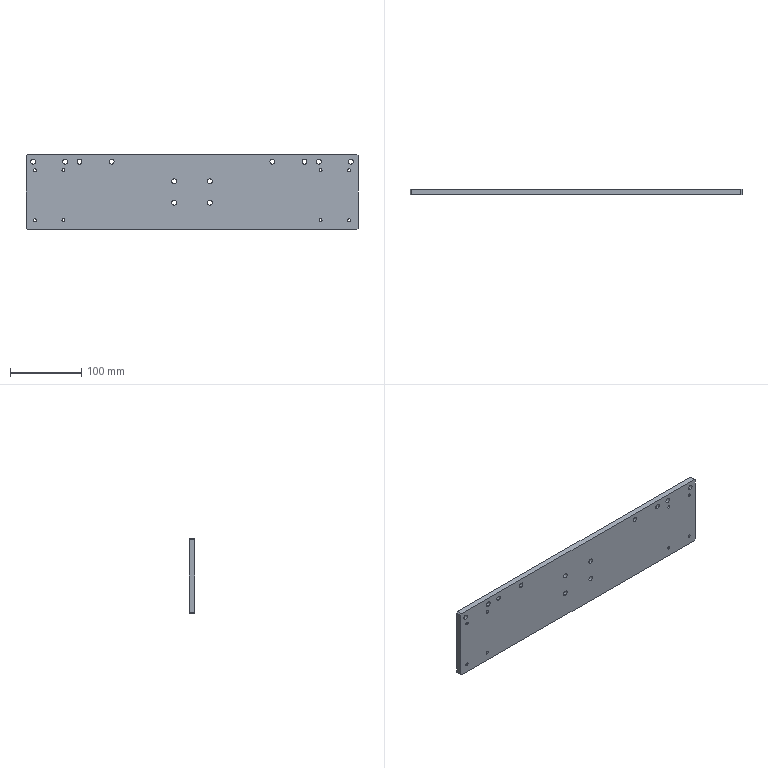Part | SolidWorks | features HoleWzd 3, Chamfer 1, Extrusion 1 | 1 solid | 50 faces | box 465 x 8 x 105 mm | volume 386163 mm3 | cylinder 40 | plane 10 | commonest cylinder face diameters 6.8 x24 4.2 x16